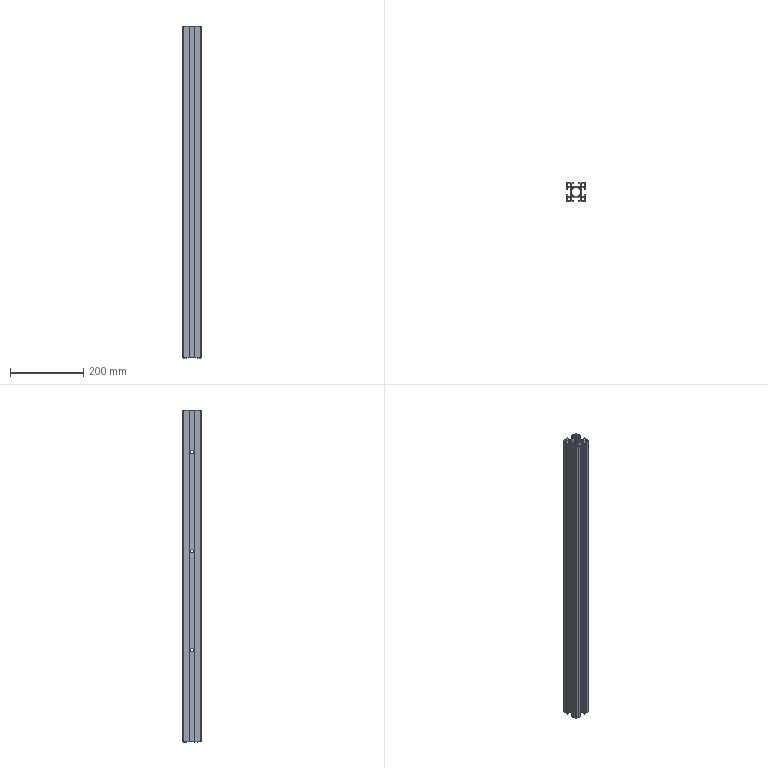Part | STEP file | DZZC_905mm | 1 solid | 154 faces | box 50 x 50 x 905 mm | volume 530917 mm3 | cylinder 96 | plane 58 | commonest cylinder face diameters 1 x24 4 x24 1.5 x16 9 x12 3.7 x8 6.7 x8